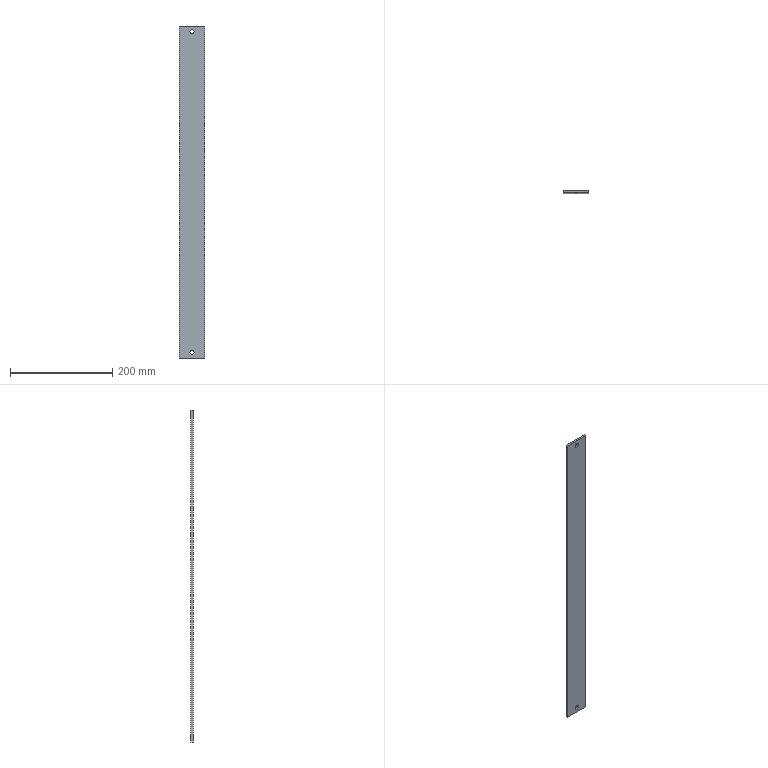Part | SolidWorks | features Extrusion 1, ICE 1 | 1 solid | 10 faces | box 50 x 5 x 650 mm | volume 161997 mm3 | plane 6 | cylinder 4 | commonest cylinder face diameters 8 x4
STEP:
#1=CARTESIAN_POINT('',(0.,0.,310.));
#2=VERTEX_POINT('',#1);
#3=CARTESIAN_POINT('',(0.,0.,318.));
#4=VERTEX_POINT('',#3);
#5=CARTESIAN_POINT('',(0.,0.,314.));
#6=DIRECTION('',(0.,1.,0.));
#7=DIRECTION('',(0.,0.,-1.));
#8=AXIS2_PLACEMENT_3D('',#5,#6,#7);
#9=CIRCLE('',#8,4.);
#10=EDGE_CURVE('',#2,#4,#9,.T.);
#11=ORIENTED_EDGE('',*,*,#10,.F.);
#12=CARTESIAN_POINT('',(0.,5.,310.));
#13=VERTEX_POINT('',#12);
#14=CARTESIAN_POINT('',(0.,0.,310.));
#15=DIRECTION('',(0.,1.,0.));
#16=VECTOR('',#15,1000.);
#17=LINE('',#14,#16);
#18=EDGE_CURVE('',#2,#13,#17,.T.);
#19=ORIENTED_EDGE('',*,*,#18,.T.);
#20=CARTESIAN_POINT('',(0.,5.,318.));
#21=VERTEX_POINT('',#20);
#22=CARTESIAN_POINT('',(0.,5.,314.));
#23=DIRECTION('',(0.,1.,0.));
#24=DIRECTION('',(0.,0.,-1.));
#25=AXIS2_PLACEMENT_3D('',#22,#23,#24);
#26=CIRCLE('',#25,4.);
#27=EDGE_CURVE('',#13,#21,#26,.T.);
#28=ORIENTED_EDGE('',*,*,#27,.T.);
#29=CARTESIAN_POINT('',(0.,0.,318.));
#30=DIRECTION('',(0.,1.,0.));
#31=VECTOR('',#30,1000.);
#32=LINE('',#29,#31);
#33=EDGE_CURVE('',#4,#21,#32,.T.);
#34=ORIENTED_EDGE('',*,*,#33,.F.);
#35=EDGE_LOOP('',(#11,#19,#28,#34));
#36=FACE_OUTER_BOUND('',#35,.T.);
#37=CARTESIAN_POINT('',(0.,0.,314.));
#38=DIRECTION('',(0.,1.,0.));
#39=DIRECTION('',(0.,0.,1.));
#40=AXIS2_PLACEMENT_3D('',#37,#38,#39);
#41=CYLINDRICAL_SURFACE('',#40,4.);
#42=ADVANCED_FACE('',(#36),#41,.F.);
#43=CARTESIAN_POINT('',(0.,0.,-318.));
#44=VERTEX_POINT('',#43);
#45=CARTESIAN_POINT('',(0.,0.,-310.));
#46=VERTEX_POINT('',#45);
#47=CARTESIAN_POINT('',(0.,0.,-314.));
#48=DIRECTION('',(0.,1.,0.));
#49=DIRECTION('',(0.,0.,1.));
#50=AXIS2_PLACEMENT_3D('',#47,#48,#49);
#51=CIRCLE('',#50,4.);
#52=EDGE_CURVE('',#44,#46,#51,.T.);
#53=ORIENTED_EDGE('',*,*,#52,.F.);
#54=CARTESIAN_POINT('',(0.,5.,-318.));
#55=VERTEX_POINT('',#54);
#56=CARTESIAN_POINT('',(0.,0.,-318.));
#57=DIRECTION('',(0.,1.,0.));
#58=VECTOR('',#57,1000.);
#59=LINE('',#56,#58);
#60=EDGE_CURVE('',#44,#55,#59,.T.);
#61=ORIENTED_EDGE('',*,*,#60,.T.);
#62=CARTESIAN_POINT('',(0.,5.,-310.));
#63=VERTEX_POINT('',#62);
#64=CARTESIAN_POINT('',(0.,5.,-314.));
#65=DIRECTION('',(0.,1.,0.));
#66=DIRECTION('',(0.,0.,1.));
#67=AXIS2_PLACEMENT_3D('',#64,#65,#66);
#68=CIRCLE('',#67,4.);
#69=EDGE_CURVE('',#55,#63,#68,.T.);
#70=ORIENTED_EDGE('',*,*,#69,.T.);
#71=CARTESIAN_POINT('',(0.,0.,-310.));
#72=DIRECTION('',(0.,1.,0.));
#73=VECTOR('',#72,1000.);
#74=LINE('',#71,#73);
#75=EDGE_CURVE('',#46,#63,#74,.T.);
#76=ORIENTED_EDGE('',*,*,#75,.F.);
#77=EDGE_LOOP('',(#53,#61,#70,#76));
#78=FACE_OUTER_BOUND('',#77,.T.);
#79=CARTESIAN_POINT('',(0.,0.,-314.));
#80=DIRECTION('',(0.,1.,0.));
#81=DIRECTION('',(0.,0.,1.));
#82=AXIS2_PLACEMENT_3D('',#79,#80,#81);
#83=CYLINDRICAL_SURFACE('',#82,4.);
#84=ADVANCED_FACE('',(#78),#83,.F.);
#85=CARTESIAN_POINT('',(25.,0.,325.));
#86=VERTEX_POINT('',#85);
#87=CARTESIAN_POINT('',(25.,0.,-325.));
#88=VERTEX_POINT('',#87);
#89=CARTESIAN_POINT('',(25.,0.,-325.));
#90=DIRECTION('',(0.,0.,-1.));
#91=VECTOR('',#90,1000.);
#92=LINE('',#89,#91);
#93=EDGE_CURVE('',#86,#88,#92,.T.);
#94=ORIENTED_EDGE('',*,*,#93,.T.);
#95=CARTESIAN_POINT('',(25.,5.,-325.));
#96=VERTEX_POINT('',#95);
#97=CARTESIAN_POINT('',(25.,5.,-325.));
#98=DIRECTION('',(0.,-1.,0.));
#99=VECTOR('',#98,1000.);
#100=LINE('',#97,#99);
#101=EDGE_CURVE('',#96,#88,#100,.T.);
#102=ORIENTED_EDGE('',*,*,#101,.F.);
#103=CARTESIAN_POINT('',(25.,5.,325.));
#104=VERTEX_POINT('',#103);
#105=CARTESIAN_POINT('',(25.,5.,-325.));
#106=DIRECTION('',(0.,0.,-1.));
#107=VECTOR('',#106,1000.);
#108=LINE('',#105,#107);
#109=EDGE_CURVE('',#104,#96,#108,.T.);
#110=ORIENTED_EDGE('',*,*,#109,.F.);
#111=CARTESIAN_POINT('',(25.,5.,325.));
#112=DIRECTION('',(0.,-1.,0.));
#113=VECTOR('',#112,1000.);
#114=LINE('',#111,#113);
#115=EDGE_CURVE('',#104,#86,#114,.T.);
#116=ORIENTED_EDGE('',*,*,#115,.T.);
#117=EDGE_LOOP('',(#94,#102,#110,#116));
#118=FACE_OUTER_BOUND('',#117,.T.);
#119=CARTESIAN_POINT('',(25.,5.,-325.));
#120=DIRECTION('',(-1.,0.,0.));
#121=DIRECTION('',(0.,0.,1.));
#122=AXIS2_PLACEMENT_3D('',#119,#120,#121);
#123=PLANE('',#122);
#124=ADVANCED_FACE('',(#118),#123,.F.);
#125=CARTESIAN_POINT('',(-25.,0.,-325.));
#126=VERTEX_POINT('',#125);
#127=CARTESIAN_POINT('',(-25.,0.,-325.));
#128=DIRECTION('',(-1.,0.,0.));
#129=VECTOR('',#128,1000.);
#130=LINE('',#127,#129);
#131=EDGE_CURVE('',#88,#126,#130,.T.);
#132=ORIENTED_EDGE('',*,*,#131,.T.);
#133=CARTESIAN_POINT('',(-25.,5.,-325.));
#134=VERTEX_POINT('',#133);
#135=CARTESIAN_POINT('',(-25.,5.,-325.));
#136=DIRECTION('',(0.,-1.,0.));
#137=VECTOR('',#136,1000.);
#138=LINE('',#135,#137);
#139=EDGE_CURVE('',#134,#126,#138,.T.);
#140=ORIENTED_EDGE('',*,*,#139,.F.);
#141=CARTESIAN_POINT('',(-25.,5.,-325.));
#142=DIRECTION('',(-1.,0.,0.));
#143=VECTOR('',#142,1000.);
#144=LINE('',#141,#143);
#145=EDGE_CURVE('',#96,#134,#144,.T.);
#146=ORIENTED_EDGE('',*,*,#145,.F.);
#147=ORIENTED_EDGE('',*,*,#101,.T.);
#148=EDGE_LOOP('',(#132,#140,#146,#147));
#149=FACE_OUTER_BOUND('',#148,.T.);
#150=CARTESIAN_POINT('',(-25.,5.,-325.));
#151=DIRECTION('',(0.,0.,1.));
#152=DIRECTION('',(1.,0.,0.));
#153=AXIS2_PLACEMENT_3D('',#150,#151,#152);
#154=PLANE('',#153);
#155=ADVANCED_FACE('',(#149),#154,.F.);
#156=CARTESIAN_POINT('',(-25.,0.,325.));
#157=VERTEX_POINT('',#156);
#158=CARTESIAN_POINT('',(-25.,0.,-325.));
#159=DIRECTION('',(0.,0.,1.));
#160=VECTOR('',#159,1000.);
#161=LINE('',#158,#160);
#162=EDGE_CURVE('',#126,#157,#161,.T.);
#163=ORIENTED_EDGE('',*,*,#162,.T.);
#164=CARTESIAN_POINT('',(-25.,5.,325.));
#165=VERTEX_POINT('',#164);
#166=CARTESIAN_POINT('',(-25.,5.,325.));
#167=DIRECTION('',(0.,-1.,0.));
#168=VECTOR('',#167,1000.);
#169=LINE('',#166,#168);
#170=EDGE_CURVE('',#165,#157,#169,.T.);
#171=ORIENTED_EDGE('',*,*,#170,.F.);
#172=CARTESIAN_POINT('',(-25.,5.,-325.));
#173=DIRECTION('',(0.,0.,1.));
#174=VECTOR('',#173,1000.);
#175=LINE('',#172,#174);
#176=EDGE_CURVE('',#134,#165,#175,.T.);
#177=ORIENTED_EDGE('',*,*,#176,.F.);
#178=ORIENTED_EDGE('',*,*,#139,.T.);
#179=EDGE_LOOP('',(#163,#171,#177,#178));
#180=FACE_OUTER_BOUND('',#179,.T.);
#181=CARTESIAN_POINT('',(-25.,5.,-325.));
#182=DIRECTION('',(1.,0.,0.));
#183=DIRECTION('',(0.,0.,-1.));
#184=AXIS2_PLACEMENT_3D('',#181,#182,#183);
#185=PLANE('',#184);
#186=ADVANCED_FACE('',(#180),#185,.F.);
#187=CARTESIAN_POINT('',(-25.,0.,325.));
#188=DIRECTION('',(1.,0.,0.));
#189=VECTOR('',#188,1000.);
#190=LINE('',#187,#189);
#191=EDGE_CURVE('',#157,#86,#190,.T.);
#192=ORIENTED_EDGE('',*,*,#191,.T.);
#193=ORIENTED_EDGE('',*,*,#115,.F.);
#194=CARTESIAN_POINT('',(-25.,5.,325.));
#195=DIRECTION('',(1.,0.,0.));
#196=VECTOR('',#195,1000.);
#197=LINE('',#194,#196);
#198=EDGE_CURVE('',#165,#104,#197,.T.);
#199=ORIENTED_EDGE('',*,*,#198,.F.);
#200=ORIENTED_EDGE('',*,*,#170,.T.);
#201=EDGE_LOOP('',(#192,#193,#199,#200));
#202=FACE_OUTER_BOUND('',#201,.T.);
#203=CARTESIAN_POINT('',(-25.,5.,325.));
#204=DIRECTION('',(0.,0.,-1.));
#205=DIRECTION('',(-1.,0.,0.));
#206=AXIS2_PLACEMENT_3D('',#203,#204,#205);
#207=PLANE('',#206);
#208=ADVANCED_FACE('',(#202),#207,.F.);
#209=CARTESIAN_POINT('',(0.,5.,314.));
#210=DIRECTION('',(0.,1.,0.));
#211=DIRECTION('',(0.,0.,-1.));
#212=AXIS2_PLACEMENT_3D('',#209,#210,#211);
#213=CIRCLE('',#212,4.);
#214=EDGE_CURVE('',#21,#13,#213,.T.);
#215=ORIENTED_EDGE('',*,*,#214,.F.);
#216=ORIENTED_EDGE('',*,*,#27,.F.);
#217=EDGE_LOOP('',(#215,#216));
#218=FACE_BOUND('',#217,.T.);
#219=CARTESIAN_POINT('',(0.,5.,-314.));
#220=DIRECTION('',(0.,1.,0.));
#221=DIRECTION('',(0.,0.,1.));
#222=AXIS2_PLACEMENT_3D('',#219,#220,#221);
#223=CIRCLE('',#222,4.);
#224=EDGE_CURVE('',#63,#55,#223,.T.);
#225=ORIENTED_EDGE('',*,*,#224,.F.);
#226=ORIENTED_EDGE('',*,*,#69,.F.);
#227=EDGE_LOOP('',(#225,#226));
#228=FACE_BOUND('',#227,.T.);
#229=ORIENTED_EDGE('',*,*,#109,.T.);
#230=ORIENTED_EDGE('',*,*,#145,.T.);
#231=ORIENTED_EDGE('',*,*,#176,.T.);
#232=ORIENTED_EDGE('',*,*,#198,.T.);
#233=EDGE_LOOP('',(#229,#230,#231,#232));
#234=FACE_OUTER_BOUND('',#233,.T.);
#235=CARTESIAN_POINT('',(0.,5.,0.));
#236=DIRECTION('',(0.,1.,0.));
#237=DIRECTION('',(0.,0.,1.));
#238=AXIS2_PLACEMENT_3D('',#235,#236,#237);
#239=PLANE('',#238);
#240=ADVANCED_FACE('',(#218,#228,#234),#239,.T.);
#241=CARTESIAN_POINT('',(0.,0.,314.));
#242=DIRECTION('',(0.,1.,0.));
#243=DIRECTION('',(0.,0.,-1.));
#244=AXIS2_PLACEMENT_3D('',#241,#242,#243);
#245=CIRCLE('',#244,4.);
#246=EDGE_CURVE('',#4,#2,#245,.T.);
#247=ORIENTED_EDGE('',*,*,#246,.T.);
#248=ORIENTED_EDGE('',*,*,#10,.T.);
#249=EDGE_LOOP('',(#247,#248));
#250=FACE_BOUND('',#249,.T.);
#251=CARTESIAN_POINT('',(0.,0.,-314.));
#252=DIRECTION('',(0.,1.,0.));
#253=DIRECTION('',(0.,0.,1.));
#254=AXIS2_PLACEMENT_3D('',#251,#252,#253);
#255=CIRCLE('',#254,4.);
#256=EDGE_CURVE('',#46,#44,#255,.T.);
#257=ORIENTED_EDGE('',*,*,#256,.T.);
#258=ORIENTED_EDGE('',*,*,#52,.T.);
#259=EDGE_LOOP('',(#257,#258));
#260=FACE_BOUND('',#259,.T.);
#261=ORIENTED_EDGE('',*,*,#93,.F.);
#262=ORIENTED_EDGE('',*,*,#191,.F.);
#263=ORIENTED_EDGE('',*,*,#162,.F.);
#264=ORIENTED_EDGE('',*,*,#131,.F.);
#265=EDGE_LOOP('',(#261,#262,#263,#264));
#266=FACE_OUTER_BOUND('',#265,.T.);
#267=CARTESIAN_POINT('',(0.,0.,0.));
#268=DIRECTION('',(0.,1.,0.));
#269=DIRECTION('',(0.,0.,1.));
#270=AXIS2_PLACEMENT_3D('',#267,#268,#269);
#271=PLANE('',#270);
#272=ADVANCED_FACE('',(#250,#260,#266),#271,.F.);
#273=ORIENTED_EDGE('',*,*,#60,.F.);
#274=ORIENTED_EDGE('',*,*,#256,.F.);
#275=ORIENTED_EDGE('',*,*,#75,.T.);
#276=ORIENTED_EDGE('',*,*,#224,.T.);
#277=EDGE_LOOP('',(#273,#274,#275,#276));
#278=FACE_OUTER_BOUND('',#277,.T.);
#279=CARTESIAN_POINT('',(0.,0.,-314.));
#280=DIRECTION('',(0.,1.,0.));
#281=DIRECTION('',(0.,0.,1.));
#282=AXIS2_PLACEMENT_3D('',#279,#280,#281);
#283=CYLINDRICAL_SURFACE('',#282,4.);
#284=ADVANCED_FACE('',(#278),#283,.F.);
#285=ORIENTED_EDGE('',*,*,#18,.F.);
#286=ORIENTED_EDGE('',*,*,#246,.F.);
#287=ORIENTED_EDGE('',*,*,#33,.T.);
#288=ORIENTED_EDGE('',*,*,#214,.T.);
#289=EDGE_LOOP('',(#285,#286,#287,#288));
#290=FACE_OUTER_BOUND('',#289,.T.);
#291=CARTESIAN_POINT('',(0.,0.,314.));
#292=DIRECTION('',(0.,1.,0.));
#293=DIRECTION('',(0.,0.,1.));
#294=AXIS2_PLACEMENT_3D('',#291,#292,#293);
#295=CYLINDRICAL_SURFACE('',#294,4.);
#296=ADVANCED_FACE('',(#290),#295,.F.);
#297=CLOSED_SHELL('',(#42,#84,#124,#155,#186,#208,#240,#272,#284,#296));
#298=MANIFOLD_SOLID_BREP('',#297);
#299=CARTESIAN_POINT('',(0.,0.,0.));
#300=DIRECTION('',(0.,0.,1.));
#301=DIRECTION('',(1.,0.,0.));
#302=AXIS2_PLACEMENT_3D('',#299,#300,#301);
#303=(LENGTH_UNIT()NAMED_UNIT(*)SI_UNIT(.MILLI.,.METRE.));
#304=UNCERTAINTY_MEASURE_WITH_UNIT(LENGTH_MEASURE(0.00001),#303,'','');
#305=(NAMED_UNIT(*)PLANE_ANGLE_UNIT()SI_UNIT($,.RADIAN.));
#306=(NAMED_UNIT(*)SI_UNIT($,.STERADIAN.)SOLID_ANGLE_UNIT());
#307=(GEOMETRIC_REPRESENTATION_CONTEXT(3)GLOBAL_UNCERTAINTY_ASSIGNED_CONTEXT((#304))GLOBAL_UNIT_ASSIGNED_CONTEXT((#303,#305,#306))REPRESENTATION_CONTEXT('',''));
#308=ADVANCED_BREP_SHAPE_REPRESENTATION('',(#298,#302),#307);